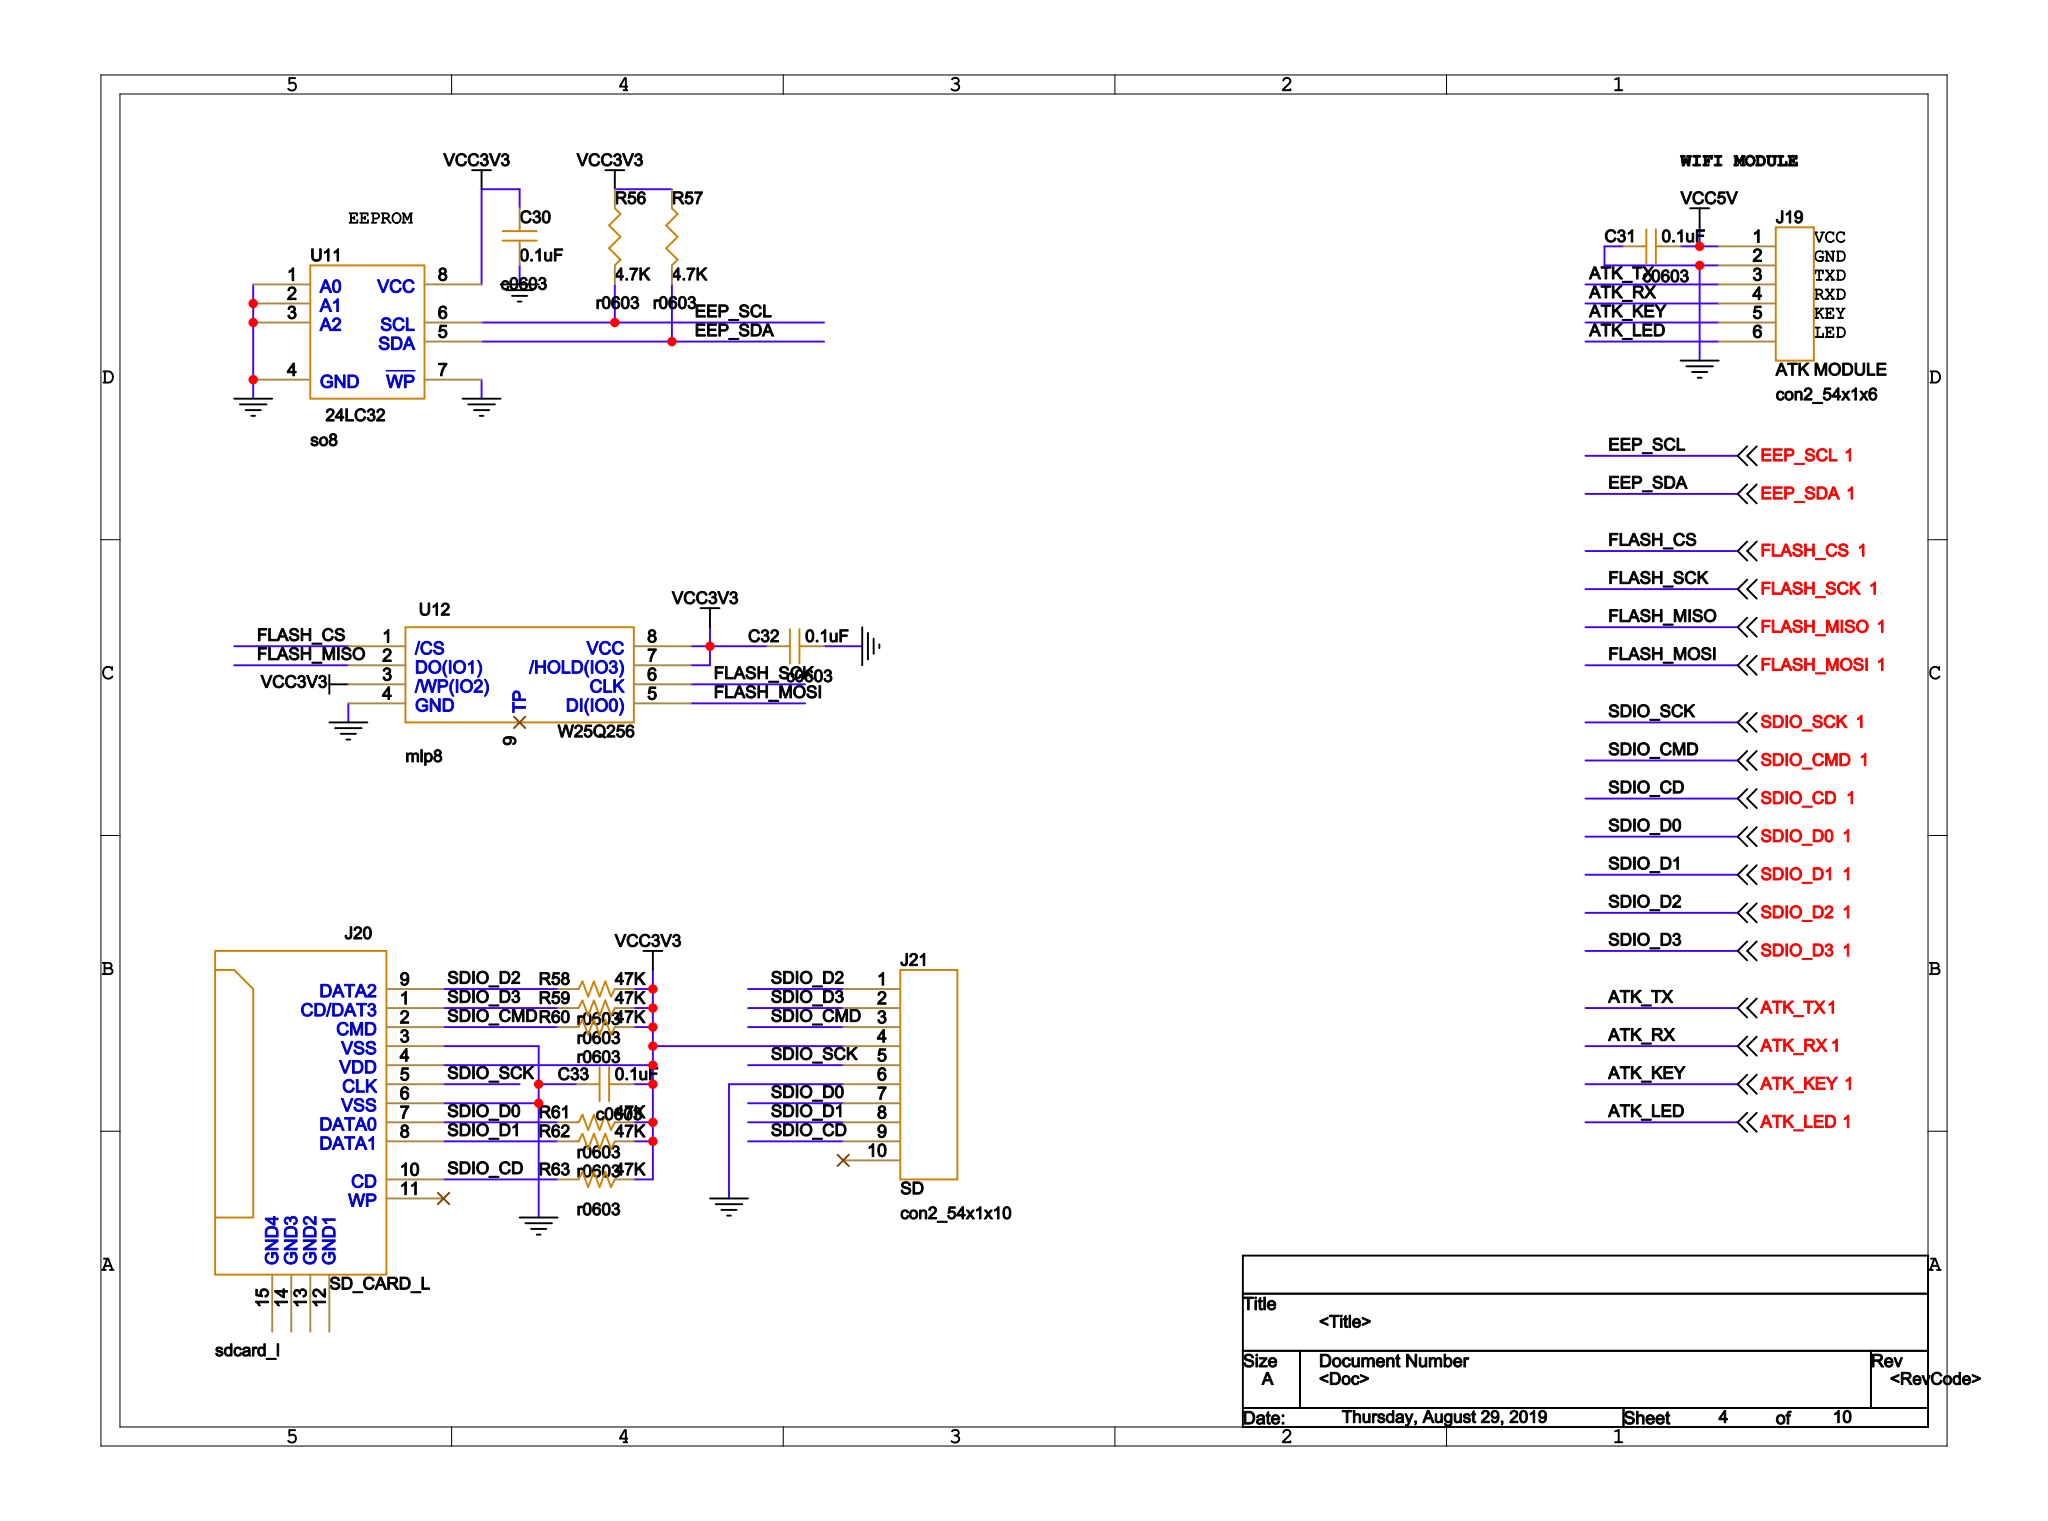Circuit board | Cadence Allegro | 380 parts | 375 nets | one sheet of the schematic
Parts on this sheet (reference | value | footprint):
C30 | 0.1uF | C0603
C31 | 0.1uF | C0603
C32 | 0.1uF | C0603
C33 | 0.1uF | C0603
J19 | ATK MODULE | CON2_54X1X6
J20 | SD_CARD_L | SDCARD_L
J21 | SD | CON2_54X1X10
R56 | 4.7K | R0603
R57 | 4.7K | R0603
R58 | 47K | R0603
R59 | 47K | R0603
R60 | 47K | R0603
R61 | 47K | R0603
R62 | 47K | R0603
R63 | 47K | R0603
U11 | 24LC32 | SO8
U12 | W25Q256 | MLP8
Nets of these parts (net: part-pin ...):
GND: C30-2 C31-1 C32-2 C33-1 J19-2 J20-3 J20-6 J21-6 U11-1 U11-2 U11-3 U11-4 U11-7 U12-4
VCC3V3: C30-1 C32-1 C33-2 J20-4 J21-4 R56-1 R57-1 R58-2 R59-2 R60-2 R61-2 R62-2 R63-2 U11-8 U12-3 U12-7 U12-8
SDIO_CD: J20-10 J21-9 R63-1
SDIO_D3: J20-1 J21-2 R59-1
SDIO_SCK: J20-5 J21-5
SDIO_CMD: J20-2 J21-3 R60-1
SDIO_D0: J20-7 J21-7 R61-1
SDIO_D1: J20-8 J21-8 R62-1
SDIO_D2: J20-9 J21-1 R58-1
GND1: J20-12
GND2: J20-13
GND3: J20-14
GND4: J20-15
VCC5V: C31-2 J19-1
EEP_SCL: R56-2 U11-6
EEP_SDA: R57-2 U11-5
FLASH_CS: U12-1
FLASH_SCK: U12-6
FLASH_MOSI: U12-5
FLASH_MISO: U12-2
ATK_TX: J19-3
ATK_RX: J19-4
ATK_KEY: J19-5
ATK_LED: J19-6